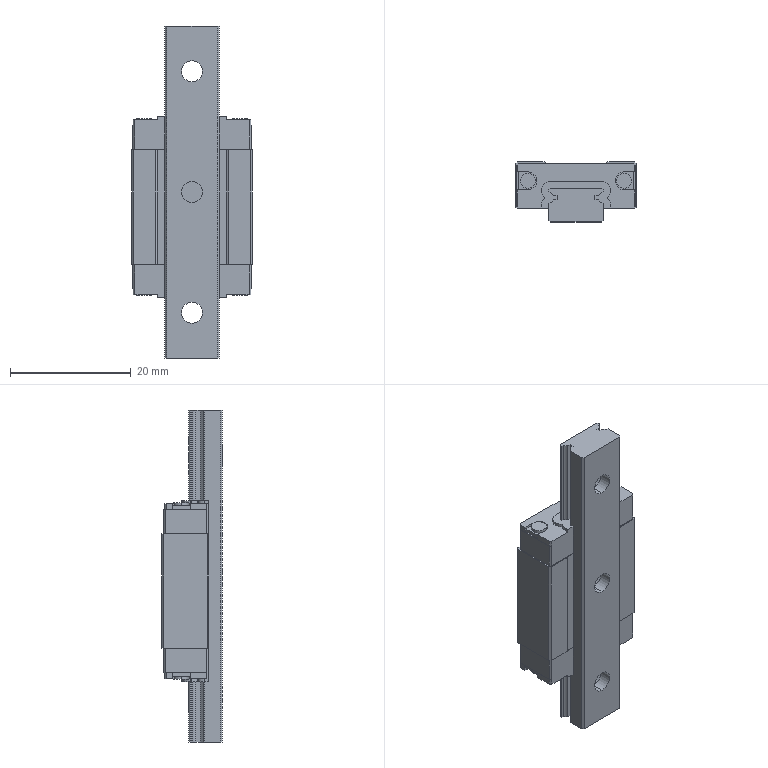Part | SolidWorks | 2 solids | 299 faces | box 20 x 10 x 55 mm | volume 5673 mm3 | plane 207 | cylinder 76 | cone 16 | commonest cylinder face diameters 2.2 x16 3 x10 2.1 x8 2.459 x8 2.5 x8 2.6 x8